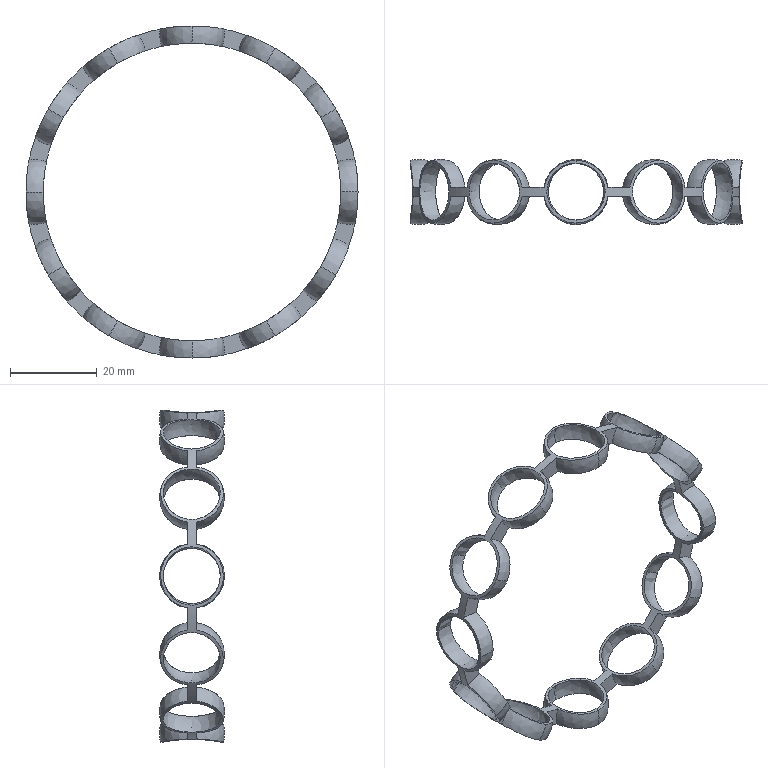Part | SolidWorks | features CirPattern 2, Extrusion 1, ICE 1, RevCut 1, Revolution 1 | 1 solid | 100 faces | box 76.5 x 15 x 76.5 mm | volume 1814 mm3 | sphere 72 | plane 24 | cylinder 4 | commonest cylinder face diameters 68.5 x2 76.5 x2